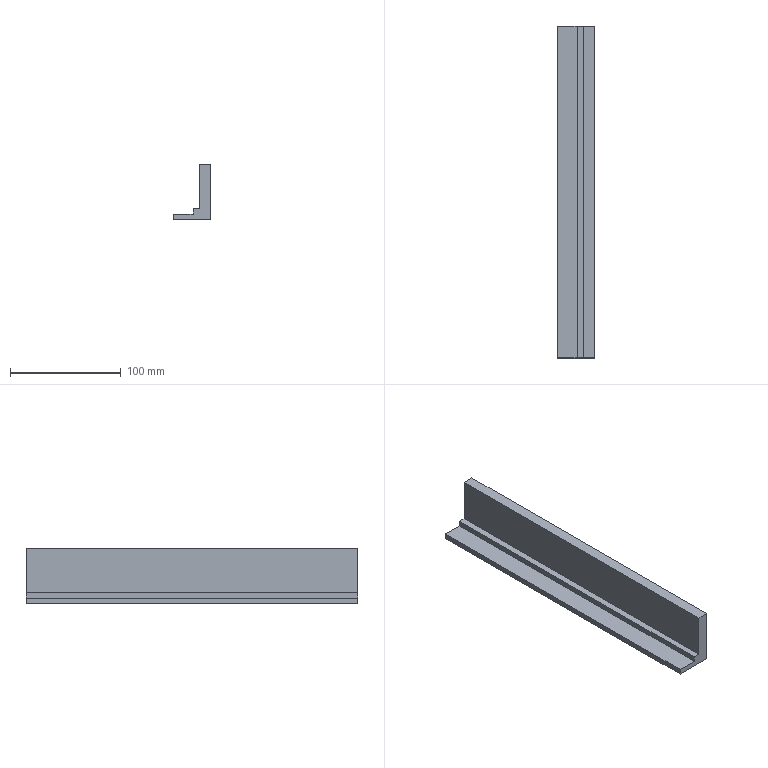Part | STEP file | Platform 1 slider plate 1 | 1 solid | 10 faces | box 34 x 300 x 50 mm | volume 195000 mm3 | plane 10
STEP:
#1=CARTESIAN_POINT('',(0.,-150.,0.));
#2=VERTEX_POINT('',#1);
#3=CARTESIAN_POINT('',(0.,-150.,5.));
#4=VERTEX_POINT('',#3);
#5=CARTESIAN_POINT('',(0.,-150.,10.));
#6=DIRECTION('',(0.,0.,1.));
#7=VECTOR('',#6,1000.);
#8=LINE('',#5,#7);
#9=EDGE_CURVE('',#2,#4,#8,.T.);
#10=ORIENTED_EDGE('',*,*,#9,.T.);
#11=CARTESIAN_POINT('',(0.,150.,5.));
#12=VERTEX_POINT('',#11);
#13=CARTESIAN_POINT('',(0.,-150.,5.));
#14=DIRECTION('',(0.,1.,0.));
#15=VECTOR('',#14,1000.);
#16=LINE('',#13,#15);
#17=EDGE_CURVE('',#4,#12,#16,.T.);
#18=ORIENTED_EDGE('',*,*,#17,.T.);
#19=CARTESIAN_POINT('',(0.,150.,0.));
#20=VERTEX_POINT('',#19);
#21=CARTESIAN_POINT('',(0.,150.,10.));
#22=DIRECTION('',(0.,0.,1.));
#23=VECTOR('',#22,1000.);
#24=LINE('',#21,#23);
#25=EDGE_CURVE('',#20,#12,#24,.T.);
#26=ORIENTED_EDGE('',*,*,#25,.F.);
#27=CARTESIAN_POINT('',(0.,150.,0.));
#28=DIRECTION('',(0.,-1.,0.));
#29=VECTOR('',#28,1000.);
#30=LINE('',#27,#29);
#31=EDGE_CURVE('',#20,#2,#30,.T.);
#32=ORIENTED_EDGE('',*,*,#31,.T.);
#33=EDGE_LOOP('',(#10,#18,#26,#32));
#34=FACE_OUTER_BOUND('',#33,.T.);
#35=CARTESIAN_POINT('',(0.,150.,10.));
#36=DIRECTION('',(1.,0.,0.));
#37=DIRECTION('',(0.,0.,-1.));
#38=AXIS2_PLACEMENT_3D('',#35,#36,#37);
#39=PLANE('',#38);
#40=ADVANCED_FACE('',(#34),#39,.F.);
#41=CARTESIAN_POINT('',(18.,150.,10.));
#42=VERTEX_POINT('',#41);
#43=CARTESIAN_POINT('',(24.,150.,10.));
#44=VERTEX_POINT('',#43);
#45=CARTESIAN_POINT('',(24.,150.,10.));
#46=DIRECTION('',(1.,0.,0.));
#47=VECTOR('',#46,1000.);
#48=LINE('',#45,#47);
#49=EDGE_CURVE('',#42,#44,#48,.T.);
#50=ORIENTED_EDGE('',*,*,#49,.F.);
#51=CARTESIAN_POINT('',(18.,-150.,10.));
#52=VERTEX_POINT('',#51);
#53=CARTESIAN_POINT('',(18.,-150.,10.));
#54=DIRECTION('',(0.,1.,0.));
#55=VECTOR('',#54,1000.);
#56=LINE('',#53,#55);
#57=EDGE_CURVE('',#52,#42,#56,.T.);
#58=ORIENTED_EDGE('',*,*,#57,.F.);
#59=CARTESIAN_POINT('',(24.,-150.,10.));
#60=VERTEX_POINT('',#59);
#61=CARTESIAN_POINT('',(24.,-150.,10.));
#62=DIRECTION('',(1.,0.,0.));
#63=VECTOR('',#62,1000.);
#64=LINE('',#61,#63);
#65=EDGE_CURVE('',#52,#60,#64,.T.);
#66=ORIENTED_EDGE('',*,*,#65,.T.);
#67=CARTESIAN_POINT('',(24.,150.,10.));
#68=DIRECTION('',(0.,-1.,0.));
#69=VECTOR('',#68,1000.);
#70=LINE('',#67,#69);
#71=EDGE_CURVE('',#44,#60,#70,.T.);
#72=ORIENTED_EDGE('',*,*,#71,.F.);
#73=EDGE_LOOP('',(#50,#58,#66,#72));
#74=FACE_OUTER_BOUND('',#73,.T.);
#75=CARTESIAN_POINT('',(24.,150.,10.));
#76=DIRECTION('',(0.,0.,-1.));
#77=DIRECTION('',(-1.,0.,0.));
#78=AXIS2_PLACEMENT_3D('',#75,#76,#77);
#79=PLANE('',#78);
#80=ADVANCED_FACE('',(#74),#79,.F.);
#81=CARTESIAN_POINT('',(24.,-150.,50.));
#82=VERTEX_POINT('',#81);
#83=CARTESIAN_POINT('',(24.,-150.,50.));
#84=DIRECTION('',(0.,0.,1.));
#85=VECTOR('',#84,1000.);
#86=LINE('',#83,#85);
#87=EDGE_CURVE('',#60,#82,#86,.T.);
#88=ORIENTED_EDGE('',*,*,#87,.T.);
#89=CARTESIAN_POINT('',(24.,150.,50.));
#90=VERTEX_POINT('',#89);
#91=CARTESIAN_POINT('',(24.,150.,50.));
#92=DIRECTION('',(0.,-1.,0.));
#93=VECTOR('',#92,1000.);
#94=LINE('',#91,#93);
#95=EDGE_CURVE('',#90,#82,#94,.T.);
#96=ORIENTED_EDGE('',*,*,#95,.F.);
#97=CARTESIAN_POINT('',(24.,150.,50.));
#98=DIRECTION('',(0.,0.,1.));
#99=VECTOR('',#98,1000.);
#100=LINE('',#97,#99);
#101=EDGE_CURVE('',#44,#90,#100,.T.);
#102=ORIENTED_EDGE('',*,*,#101,.F.);
#103=ORIENTED_EDGE('',*,*,#71,.T.);
#104=EDGE_LOOP('',(#88,#96,#102,#103));
#105=FACE_OUTER_BOUND('',#104,.T.);
#106=CARTESIAN_POINT('',(24.,150.,50.));
#107=DIRECTION('',(1.,0.,0.));
#108=DIRECTION('',(0.,0.,-1.));
#109=AXIS2_PLACEMENT_3D('',#106,#107,#108);
#110=PLANE('',#109);
#111=ADVANCED_FACE('',(#105),#110,.F.);
#112=CARTESIAN_POINT('',(34.,-150.,50.));
#113=VERTEX_POINT('',#112);
#114=CARTESIAN_POINT('',(34.,-150.,50.));
#115=DIRECTION('',(1.,0.,0.));
#116=VECTOR('',#115,1000.);
#117=LINE('',#114,#116);
#118=EDGE_CURVE('',#82,#113,#117,.T.);
#119=ORIENTED_EDGE('',*,*,#118,.T.);
#120=CARTESIAN_POINT('',(34.,150.,50.));
#121=VERTEX_POINT('',#120);
#122=CARTESIAN_POINT('',(34.,150.,50.));
#123=DIRECTION('',(0.,-1.,0.));
#124=VECTOR('',#123,1000.);
#125=LINE('',#122,#124);
#126=EDGE_CURVE('',#121,#113,#125,.T.);
#127=ORIENTED_EDGE('',*,*,#126,.F.);
#128=CARTESIAN_POINT('',(34.,150.,50.));
#129=DIRECTION('',(1.,0.,0.));
#130=VECTOR('',#129,1000.);
#131=LINE('',#128,#130);
#132=EDGE_CURVE('',#90,#121,#131,.T.);
#133=ORIENTED_EDGE('',*,*,#132,.F.);
#134=ORIENTED_EDGE('',*,*,#95,.T.);
#135=EDGE_LOOP('',(#119,#127,#133,#134));
#136=FACE_OUTER_BOUND('',#135,.T.);
#137=CARTESIAN_POINT('',(34.,150.,50.));
#138=DIRECTION('',(0.,0.,-1.));
#139=DIRECTION('',(-1.,0.,0.));
#140=AXIS2_PLACEMENT_3D('',#137,#138,#139);
#141=PLANE('',#140);
#142=ADVANCED_FACE('',(#136),#141,.F.);
#143=CARTESIAN_POINT('',(34.,-150.,0.));
#144=VERTEX_POINT('',#143);
#145=CARTESIAN_POINT('',(34.,-150.,0.));
#146=DIRECTION('',(0.,0.,-1.));
#147=VECTOR('',#146,1000.);
#148=LINE('',#145,#147);
#149=EDGE_CURVE('',#113,#144,#148,.T.);
#150=ORIENTED_EDGE('',*,*,#149,.T.);
#151=CARTESIAN_POINT('',(34.,150.,0.));
#152=VERTEX_POINT('',#151);
#153=CARTESIAN_POINT('',(34.,150.,0.));
#154=DIRECTION('',(0.,-1.,0.));
#155=VECTOR('',#154,1000.);
#156=LINE('',#153,#155);
#157=EDGE_CURVE('',#152,#144,#156,.T.);
#158=ORIENTED_EDGE('',*,*,#157,.F.);
#159=CARTESIAN_POINT('',(34.,150.,0.));
#160=DIRECTION('',(0.,0.,-1.));
#161=VECTOR('',#160,1000.);
#162=LINE('',#159,#161);
#163=EDGE_CURVE('',#121,#152,#162,.T.);
#164=ORIENTED_EDGE('',*,*,#163,.F.);
#165=ORIENTED_EDGE('',*,*,#126,.T.);
#166=EDGE_LOOP('',(#150,#158,#164,#165));
#167=FACE_OUTER_BOUND('',#166,.T.);
#168=CARTESIAN_POINT('',(34.,150.,0.));
#169=DIRECTION('',(-1.,0.,0.));
#170=DIRECTION('',(0.,0.,1.));
#171=AXIS2_PLACEMENT_3D('',#168,#169,#170);
#172=PLANE('',#171);
#173=ADVANCED_FACE('',(#167),#172,.F.);
#174=CARTESIAN_POINT('',(0.,-150.,0.));
#175=DIRECTION('',(-1.,0.,0.));
#176=VECTOR('',#175,1000.);
#177=LINE('',#174,#176);
#178=EDGE_CURVE('',#144,#2,#177,.T.);
#179=ORIENTED_EDGE('',*,*,#178,.T.);
#180=ORIENTED_EDGE('',*,*,#31,.F.);
#181=CARTESIAN_POINT('',(0.,150.,0.));
#182=DIRECTION('',(-1.,0.,0.));
#183=VECTOR('',#182,1000.);
#184=LINE('',#181,#183);
#185=EDGE_CURVE('',#152,#20,#184,.T.);
#186=ORIENTED_EDGE('',*,*,#185,.F.);
#187=ORIENTED_EDGE('',*,*,#157,.T.);
#188=EDGE_LOOP('',(#179,#180,#186,#187));
#189=FACE_OUTER_BOUND('',#188,.T.);
#190=CARTESIAN_POINT('',(0.,150.,0.));
#191=DIRECTION('',(0.,0.,1.));
#192=DIRECTION('',(1.,0.,0.));
#193=AXIS2_PLACEMENT_3D('',#190,#191,#192);
#194=PLANE('',#193);
#195=ADVANCED_FACE('',(#189),#194,.F.);
#196=ORIENTED_EDGE('',*,*,#25,.T.);
#197=CARTESIAN_POINT('',(18.,150.,5.));
#198=VERTEX_POINT('',#197);
#199=CARTESIAN_POINT('',(0.,150.,5.));
#200=DIRECTION('',(-1.,0.,0.));
#201=VECTOR('',#200,1000.);
#202=LINE('',#199,#201);
#203=EDGE_CURVE('',#198,#12,#202,.T.);
#204=ORIENTED_EDGE('',*,*,#203,.F.);
#205=CARTESIAN_POINT('',(18.,150.,10.));
#206=DIRECTION('',(0.,0.,-1.));
#207=VECTOR('',#206,1000.);
#208=LINE('',#205,#207);
#209=EDGE_CURVE('',#42,#198,#208,.T.);
#210=ORIENTED_EDGE('',*,*,#209,.F.);
#211=ORIENTED_EDGE('',*,*,#49,.T.);
#212=ORIENTED_EDGE('',*,*,#101,.T.);
#213=ORIENTED_EDGE('',*,*,#132,.T.);
#214=ORIENTED_EDGE('',*,*,#163,.T.);
#215=ORIENTED_EDGE('',*,*,#185,.T.);
#216=EDGE_LOOP('',(#196,#204,#210,#211,#212,#213,#214,#215));
#217=FACE_OUTER_BOUND('',#216,.T.);
#218=CARTESIAN_POINT('',(0.,150.,0.));
#219=DIRECTION('',(0.,-1.,0.));
#220=DIRECTION('',(0.,0.,-1.));
#221=AXIS2_PLACEMENT_3D('',#218,#219,#220);
#222=PLANE('',#221);
#223=ADVANCED_FACE('',(#217),#222,.F.);
#224=CARTESIAN_POINT('',(18.,-150.,5.));
#225=VERTEX_POINT('',#224);
#226=CARTESIAN_POINT('',(0.,-150.,5.));
#227=DIRECTION('',(-1.,0.,0.));
#228=VECTOR('',#227,1000.);
#229=LINE('',#226,#228);
#230=EDGE_CURVE('',#225,#4,#229,.T.);
#231=ORIENTED_EDGE('',*,*,#230,.T.);
#232=ORIENTED_EDGE('',*,*,#9,.F.);
#233=ORIENTED_EDGE('',*,*,#178,.F.);
#234=ORIENTED_EDGE('',*,*,#149,.F.);
#235=ORIENTED_EDGE('',*,*,#118,.F.);
#236=ORIENTED_EDGE('',*,*,#87,.F.);
#237=ORIENTED_EDGE('',*,*,#65,.F.);
#238=CARTESIAN_POINT('',(18.,-150.,10.));
#239=DIRECTION('',(0.,0.,-1.));
#240=VECTOR('',#239,1000.);
#241=LINE('',#238,#240);
#242=EDGE_CURVE('',#52,#225,#241,.T.);
#243=ORIENTED_EDGE('',*,*,#242,.T.);
#244=EDGE_LOOP('',(#231,#232,#233,#234,#235,#236,#237,#243));
#245=FACE_OUTER_BOUND('',#244,.T.);
#246=CARTESIAN_POINT('',(0.,-150.,0.));
#247=DIRECTION('',(0.,-1.,0.));
#248=DIRECTION('',(0.,0.,-1.));
#249=AXIS2_PLACEMENT_3D('',#246,#247,#248);
#250=PLANE('',#249);
#251=ADVANCED_FACE('',(#245),#250,.T.);
#252=ORIENTED_EDGE('',*,*,#203,.T.);
#253=ORIENTED_EDGE('',*,*,#17,.F.);
#254=ORIENTED_EDGE('',*,*,#230,.F.);
#255=CARTESIAN_POINT('',(18.,-150.,5.));
#256=DIRECTION('',(0.,1.,0.));
#257=VECTOR('',#256,1000.);
#258=LINE('',#255,#257);
#259=EDGE_CURVE('',#225,#198,#258,.T.);
#260=ORIENTED_EDGE('',*,*,#259,.T.);
#261=EDGE_LOOP('',(#252,#253,#254,#260));
#262=FACE_OUTER_BOUND('',#261,.T.);
#263=CARTESIAN_POINT('',(0.,-150.,5.));
#264=DIRECTION('',(0.,0.,-1.));
#265=DIRECTION('',(-1.,0.,0.));
#266=AXIS2_PLACEMENT_3D('',#263,#264,#265);
#267=PLANE('',#266);
#268=ADVANCED_FACE('',(#262),#267,.F.);
#269=ORIENTED_EDGE('',*,*,#209,.T.);
#270=ORIENTED_EDGE('',*,*,#259,.F.);
#271=ORIENTED_EDGE('',*,*,#242,.F.);
#272=ORIENTED_EDGE('',*,*,#57,.T.);
#273=EDGE_LOOP('',(#269,#270,#271,#272));
#274=FACE_OUTER_BOUND('',#273,.T.);
#275=CARTESIAN_POINT('',(18.,-150.,10.));
#276=DIRECTION('',(1.,0.,0.));
#277=DIRECTION('',(0.,0.,-1.));
#278=AXIS2_PLACEMENT_3D('',#275,#276,#277);
#279=PLANE('',#278);
#280=ADVANCED_FACE('',(#274),#279,.F.);
#281=CLOSED_SHELL('',(#40,#80,#111,#142,#173,#195,#223,#251,#268,#280));
#282=MANIFOLD_SOLID_BREP('',#281);
#283=CARTESIAN_POINT('',(0.,0.,0.));
#284=DIRECTION('',(0.,0.,1.));
#285=DIRECTION('',(1.,0.,0.));
#286=AXIS2_PLACEMENT_3D('',#283,#284,#285);
#287=(LENGTH_UNIT()NAMED_UNIT(*)SI_UNIT(.MILLI.,.METRE.));
#288=UNCERTAINTY_MEASURE_WITH_UNIT(LENGTH_MEASURE(0.00001),#287,'','');
#289=(NAMED_UNIT(*)PLANE_ANGLE_UNIT()SI_UNIT($,.RADIAN.));
#290=(NAMED_UNIT(*)SI_UNIT($,.STERADIAN.)SOLID_ANGLE_UNIT());
#291=(GEOMETRIC_REPRESENTATION_CONTEXT(3)GLOBAL_UNCERTAINTY_ASSIGNED_CONTEXT((#288))GLOBAL_UNIT_ASSIGNED_CONTEXT((#287,#289,#290))REPRESENTATION_CONTEXT('',''));
#292=ADVANCED_BREP_SHAPE_REPRESENTATION('',(#282,#286),#291);